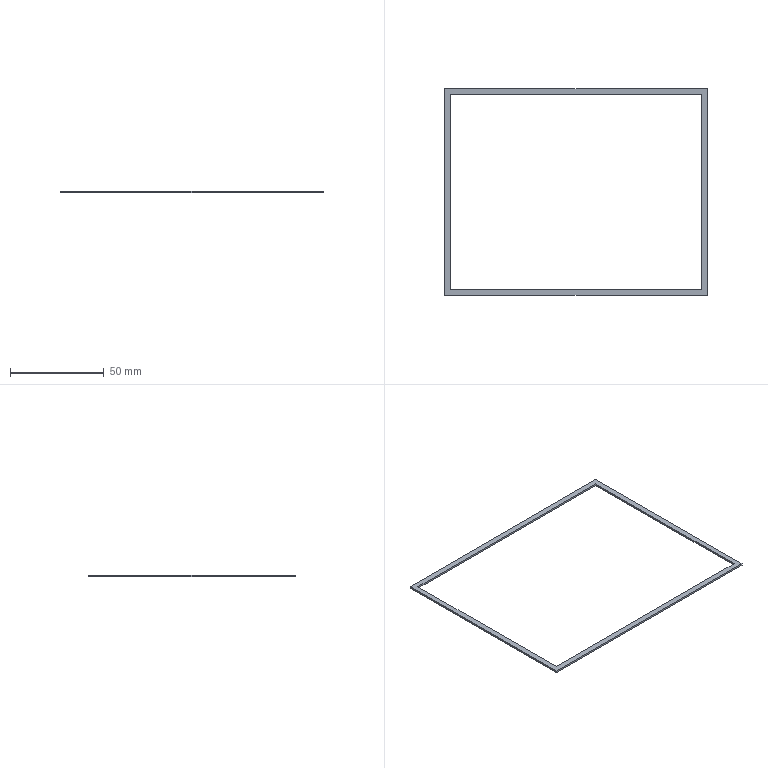Part | SolidWorks | features Extrusion 1 | 1 solid | 10 faces | box 140 x 110 x 1 mm | volume 1464 mm3 | plane 10
STEP:
#1=CARTESIAN_POINT('',(-70.,55.,0.5));
#2=VERTEX_POINT('',#1);
#3=CARTESIAN_POINT('',(-70.,-55.,0.5));
#4=VERTEX_POINT('',#3);
#5=CARTESIAN_POINT('',(-70.,55.,0.5));
#6=DIRECTION('',(0.,-1.,0.));
#7=VECTOR('',#6,1000.);
#8=LINE('',#5,#7);
#9=EDGE_CURVE('',#2,#4,#8,.T.);
#10=ORIENTED_EDGE('',*,*,#9,.F.);
#11=CARTESIAN_POINT('',(-70.,55.,-0.5));
#12=VERTEX_POINT('',#11);
#13=CARTESIAN_POINT('',(-70.,55.,-0.5));
#14=DIRECTION('',(0.,0.,1.));
#15=VECTOR('',#14,1000.);
#16=LINE('',#13,#15);
#17=EDGE_CURVE('',#12,#2,#16,.T.);
#18=ORIENTED_EDGE('',*,*,#17,.F.);
#19=CARTESIAN_POINT('',(-70.,-55.,-0.5));
#20=VERTEX_POINT('',#19);
#21=CARTESIAN_POINT('',(-70.,55.,-0.5));
#22=DIRECTION('',(0.,-1.,0.));
#23=VECTOR('',#22,1000.);
#24=LINE('',#21,#23);
#25=EDGE_CURVE('',#12,#20,#24,.T.);
#26=ORIENTED_EDGE('',*,*,#25,.T.);
#27=CARTESIAN_POINT('',(-70.,-55.,-0.5));
#28=DIRECTION('',(0.,0.,1.));
#29=VECTOR('',#28,1000.);
#30=LINE('',#27,#29);
#31=EDGE_CURVE('',#20,#4,#30,.T.);
#32=ORIENTED_EDGE('',*,*,#31,.T.);
#33=EDGE_LOOP('',(#10,#18,#26,#32));
#34=FACE_OUTER_BOUND('',#33,.T.);
#35=CARTESIAN_POINT('',(-70.,55.,-0.5));
#36=DIRECTION('',(-1.,0.,0.));
#37=DIRECTION('',(0.,0.,1.));
#38=AXIS2_PLACEMENT_3D('',#35,#36,#37);
#39=PLANE('',#38);
#40=ADVANCED_FACE('',(#34),#39,.T.);
#41=CARTESIAN_POINT('',(70.,55.,0.5));
#42=VERTEX_POINT('',#41);
#43=CARTESIAN_POINT('',(70.,55.,0.5));
#44=DIRECTION('',(-1.,0.,0.));
#45=VECTOR('',#44,1000.);
#46=LINE('',#43,#45);
#47=EDGE_CURVE('',#42,#2,#46,.T.);
#48=ORIENTED_EDGE('',*,*,#47,.F.);
#49=CARTESIAN_POINT('',(70.,55.,-0.5));
#50=VERTEX_POINT('',#49);
#51=CARTESIAN_POINT('',(70.,55.,-0.5));
#52=DIRECTION('',(0.,0.,1.));
#53=VECTOR('',#52,1000.);
#54=LINE('',#51,#53);
#55=EDGE_CURVE('',#50,#42,#54,.T.);
#56=ORIENTED_EDGE('',*,*,#55,.F.);
#57=CARTESIAN_POINT('',(70.,55.,-0.5));
#58=DIRECTION('',(-1.,0.,0.));
#59=VECTOR('',#58,1000.);
#60=LINE('',#57,#59);
#61=EDGE_CURVE('',#50,#12,#60,.T.);
#62=ORIENTED_EDGE('',*,*,#61,.T.);
#63=ORIENTED_EDGE('',*,*,#17,.T.);
#64=EDGE_LOOP('',(#48,#56,#62,#63));
#65=FACE_OUTER_BOUND('',#64,.T.);
#66=CARTESIAN_POINT('',(70.,55.,-0.5));
#67=DIRECTION('',(0.,1.,0.));
#68=DIRECTION('',(0.,0.,1.));
#69=AXIS2_PLACEMENT_3D('',#66,#67,#68);
#70=PLANE('',#69);
#71=ADVANCED_FACE('',(#65),#70,.T.);
#72=CARTESIAN_POINT('',(70.,-55.,0.5));
#73=VERTEX_POINT('',#72);
#74=CARTESIAN_POINT('',(70.,-55.,0.5));
#75=DIRECTION('',(0.,1.,0.));
#76=VECTOR('',#75,1000.);
#77=LINE('',#74,#76);
#78=EDGE_CURVE('',#73,#42,#77,.T.);
#79=ORIENTED_EDGE('',*,*,#78,.F.);
#80=CARTESIAN_POINT('',(70.,-55.,-0.5));
#81=VERTEX_POINT('',#80);
#82=CARTESIAN_POINT('',(70.,-55.,-0.5));
#83=DIRECTION('',(0.,0.,1.));
#84=VECTOR('',#83,1000.);
#85=LINE('',#82,#84);
#86=EDGE_CURVE('',#81,#73,#85,.T.);
#87=ORIENTED_EDGE('',*,*,#86,.F.);
#88=CARTESIAN_POINT('',(70.,-55.,-0.5));
#89=DIRECTION('',(0.,1.,0.));
#90=VECTOR('',#89,1000.);
#91=LINE('',#88,#90);
#92=EDGE_CURVE('',#81,#50,#91,.T.);
#93=ORIENTED_EDGE('',*,*,#92,.T.);
#94=ORIENTED_EDGE('',*,*,#55,.T.);
#95=EDGE_LOOP('',(#79,#87,#93,#94));
#96=FACE_OUTER_BOUND('',#95,.T.);
#97=CARTESIAN_POINT('',(70.,-55.,-0.5));
#98=DIRECTION('',(1.,0.,0.));
#99=DIRECTION('',(0.,0.,-1.));
#100=AXIS2_PLACEMENT_3D('',#97,#98,#99);
#101=PLANE('',#100);
#102=ADVANCED_FACE('',(#96),#101,.T.);
#103=CARTESIAN_POINT('',(-70.,-55.,0.5));
#104=DIRECTION('',(1.,0.,0.));
#105=VECTOR('',#104,1000.);
#106=LINE('',#103,#105);
#107=EDGE_CURVE('',#4,#73,#106,.T.);
#108=ORIENTED_EDGE('',*,*,#107,.F.);
#109=ORIENTED_EDGE('',*,*,#31,.F.);
#110=CARTESIAN_POINT('',(-70.,-55.,-0.5));
#111=DIRECTION('',(1.,0.,0.));
#112=VECTOR('',#111,1000.);
#113=LINE('',#110,#112);
#114=EDGE_CURVE('',#20,#81,#113,.T.);
#115=ORIENTED_EDGE('',*,*,#114,.T.);
#116=ORIENTED_EDGE('',*,*,#86,.T.);
#117=EDGE_LOOP('',(#108,#109,#115,#116));
#118=FACE_OUTER_BOUND('',#117,.T.);
#119=CARTESIAN_POINT('',(-70.,-55.,-0.5));
#120=DIRECTION('',(0.,-1.,0.));
#121=DIRECTION('',(0.,0.,-1.));
#122=AXIS2_PLACEMENT_3D('',#119,#120,#121);
#123=PLANE('',#122);
#124=ADVANCED_FACE('',(#118),#123,.T.);
#125=CARTESIAN_POINT('',(67.,52.,-0.5));
#126=VERTEX_POINT('',#125);
#127=CARTESIAN_POINT('',(-67.,52.,-0.5));
#128=VERTEX_POINT('',#127);
#129=CARTESIAN_POINT('',(67.,52.,-0.5));
#130=DIRECTION('',(-1.,0.,0.));
#131=VECTOR('',#130,1000.);
#132=LINE('',#129,#131);
#133=EDGE_CURVE('',#126,#128,#132,.T.);
#134=ORIENTED_EDGE('',*,*,#133,.T.);
#135=CARTESIAN_POINT('',(-67.,-52.,-0.5));
#136=VERTEX_POINT('',#135);
#137=CARTESIAN_POINT('',(-67.,52.,-0.5));
#138=DIRECTION('',(0.,-1.,0.));
#139=VECTOR('',#138,1000.);
#140=LINE('',#137,#139);
#141=EDGE_CURVE('',#128,#136,#140,.T.);
#142=ORIENTED_EDGE('',*,*,#141,.T.);
#143=CARTESIAN_POINT('',(67.,-52.,-0.5));
#144=VERTEX_POINT('',#143);
#145=CARTESIAN_POINT('',(-67.,-52.,-0.5));
#146=DIRECTION('',(1.,0.,0.));
#147=VECTOR('',#146,1000.);
#148=LINE('',#145,#147);
#149=EDGE_CURVE('',#136,#144,#148,.T.);
#150=ORIENTED_EDGE('',*,*,#149,.T.);
#151=CARTESIAN_POINT('',(67.,-52.,-0.5));
#152=DIRECTION('',(0.,1.,0.));
#153=VECTOR('',#152,1000.);
#154=LINE('',#151,#153);
#155=EDGE_CURVE('',#144,#126,#154,.T.);
#156=ORIENTED_EDGE('',*,*,#155,.T.);
#157=EDGE_LOOP('',(#134,#142,#150,#156));
#158=FACE_BOUND('',#157,.T.);
#159=ORIENTED_EDGE('',*,*,#25,.F.);
#160=ORIENTED_EDGE('',*,*,#61,.F.);
#161=ORIENTED_EDGE('',*,*,#92,.F.);
#162=ORIENTED_EDGE('',*,*,#114,.F.);
#163=EDGE_LOOP('',(#159,#160,#161,#162));
#164=FACE_OUTER_BOUND('',#163,.T.);
#165=CARTESIAN_POINT('',(0.,0.,-0.5));
#166=DIRECTION('',(0.,0.,1.));
#167=DIRECTION('',(1.,0.,0.));
#168=AXIS2_PLACEMENT_3D('',#165,#166,#167);
#169=PLANE('',#168);
#170=ADVANCED_FACE('',(#158,#164),#169,.F.);
#171=CARTESIAN_POINT('',(-67.,52.,0.5));
#172=VERTEX_POINT('',#171);
#173=CARTESIAN_POINT('',(-67.,-52.,0.5));
#174=VERTEX_POINT('',#173);
#175=CARTESIAN_POINT('',(-67.,52.,0.5));
#176=DIRECTION('',(0.,-1.,0.));
#177=VECTOR('',#176,1000.);
#178=LINE('',#175,#177);
#179=EDGE_CURVE('',#172,#174,#178,.T.);
#180=ORIENTED_EDGE('',*,*,#179,.F.);
#181=CARTESIAN_POINT('',(67.,52.,0.5));
#182=VERTEX_POINT('',#181);
#183=CARTESIAN_POINT('',(67.,52.,0.5));
#184=DIRECTION('',(-1.,0.,0.));
#185=VECTOR('',#184,1000.);
#186=LINE('',#183,#185);
#187=EDGE_CURVE('',#182,#172,#186,.T.);
#188=ORIENTED_EDGE('',*,*,#187,.F.);
#189=CARTESIAN_POINT('',(67.,-52.,0.5));
#190=VERTEX_POINT('',#189);
#191=CARTESIAN_POINT('',(67.,-52.,0.5));
#192=DIRECTION('',(0.,1.,0.));
#193=VECTOR('',#192,1000.);
#194=LINE('',#191,#193);
#195=EDGE_CURVE('',#190,#182,#194,.T.);
#196=ORIENTED_EDGE('',*,*,#195,.F.);
#197=CARTESIAN_POINT('',(-67.,-52.,0.5));
#198=DIRECTION('',(1.,0.,0.));
#199=VECTOR('',#198,1000.);
#200=LINE('',#197,#199);
#201=EDGE_CURVE('',#174,#190,#200,.T.);
#202=ORIENTED_EDGE('',*,*,#201,.F.);
#203=EDGE_LOOP('',(#180,#188,#196,#202));
#204=FACE_BOUND('',#203,.T.);
#205=ORIENTED_EDGE('',*,*,#9,.T.);
#206=ORIENTED_EDGE('',*,*,#107,.T.);
#207=ORIENTED_EDGE('',*,*,#78,.T.);
#208=ORIENTED_EDGE('',*,*,#47,.T.);
#209=EDGE_LOOP('',(#205,#206,#207,#208));
#210=FACE_OUTER_BOUND('',#209,.T.);
#211=CARTESIAN_POINT('',(0.,0.,0.5));
#212=DIRECTION('',(0.,0.,1.));
#213=DIRECTION('',(1.,0.,0.));
#214=AXIS2_PLACEMENT_3D('',#211,#212,#213);
#215=PLANE('',#214);
#216=ADVANCED_FACE('',(#204,#210),#215,.T.);
#217=ORIENTED_EDGE('',*,*,#179,.T.);
#218=CARTESIAN_POINT('',(-67.,-52.,-0.5));
#219=DIRECTION('',(0.,0.,1.));
#220=VECTOR('',#219,1000.);
#221=LINE('',#218,#220);
#222=EDGE_CURVE('',#136,#174,#221,.T.);
#223=ORIENTED_EDGE('',*,*,#222,.F.);
#224=ORIENTED_EDGE('',*,*,#141,.F.);
#225=CARTESIAN_POINT('',(-67.,52.,-0.5));
#226=DIRECTION('',(0.,0.,1.));
#227=VECTOR('',#226,1000.);
#228=LINE('',#225,#227);
#229=EDGE_CURVE('',#128,#172,#228,.T.);
#230=ORIENTED_EDGE('',*,*,#229,.T.);
#231=EDGE_LOOP('',(#217,#223,#224,#230));
#232=FACE_OUTER_BOUND('',#231,.T.);
#233=CARTESIAN_POINT('',(-67.,52.,-0.5));
#234=DIRECTION('',(-1.,0.,0.));
#235=DIRECTION('',(0.,0.,1.));
#236=AXIS2_PLACEMENT_3D('',#233,#234,#235);
#237=PLANE('',#236);
#238=ADVANCED_FACE('',(#232),#237,.F.);
#239=ORIENTED_EDGE('',*,*,#187,.T.);
#240=ORIENTED_EDGE('',*,*,#229,.F.);
#241=ORIENTED_EDGE('',*,*,#133,.F.);
#242=CARTESIAN_POINT('',(67.,52.,-0.5));
#243=DIRECTION('',(0.,0.,1.));
#244=VECTOR('',#243,1000.);
#245=LINE('',#242,#244);
#246=EDGE_CURVE('',#126,#182,#245,.T.);
#247=ORIENTED_EDGE('',*,*,#246,.T.);
#248=EDGE_LOOP('',(#239,#240,#241,#247));
#249=FACE_OUTER_BOUND('',#248,.T.);
#250=CARTESIAN_POINT('',(67.,52.,-0.5));
#251=DIRECTION('',(0.,1.,0.));
#252=DIRECTION('',(0.,0.,1.));
#253=AXIS2_PLACEMENT_3D('',#250,#251,#252);
#254=PLANE('',#253);
#255=ADVANCED_FACE('',(#249),#254,.F.);
#256=ORIENTED_EDGE('',*,*,#195,.T.);
#257=ORIENTED_EDGE('',*,*,#246,.F.);
#258=ORIENTED_EDGE('',*,*,#155,.F.);
#259=CARTESIAN_POINT('',(67.,-52.,-0.5));
#260=DIRECTION('',(0.,0.,1.));
#261=VECTOR('',#260,1000.);
#262=LINE('',#259,#261);
#263=EDGE_CURVE('',#144,#190,#262,.T.);
#264=ORIENTED_EDGE('',*,*,#263,.T.);
#265=EDGE_LOOP('',(#256,#257,#258,#264));
#266=FACE_OUTER_BOUND('',#265,.T.);
#267=CARTESIAN_POINT('',(67.,-52.,-0.5));
#268=DIRECTION('',(1.,0.,0.));
#269=DIRECTION('',(0.,0.,-1.));
#270=AXIS2_PLACEMENT_3D('',#267,#268,#269);
#271=PLANE('',#270);
#272=ADVANCED_FACE('',(#266),#271,.F.);
#273=ORIENTED_EDGE('',*,*,#201,.T.);
#274=ORIENTED_EDGE('',*,*,#263,.F.);
#275=ORIENTED_EDGE('',*,*,#149,.F.);
#276=ORIENTED_EDGE('',*,*,#222,.T.);
#277=EDGE_LOOP('',(#273,#274,#275,#276));
#278=FACE_OUTER_BOUND('',#277,.T.);
#279=CARTESIAN_POINT('',(-67.,-52.,-0.5));
#280=DIRECTION('',(0.,-1.,0.));
#281=DIRECTION('',(0.,0.,-1.));
#282=AXIS2_PLACEMENT_3D('',#279,#280,#281);
#283=PLANE('',#282);
#284=ADVANCED_FACE('',(#278),#283,.F.);
#285=CLOSED_SHELL('',(#40,#71,#102,#124,#170,#216,#238,#255,#272,#284));
#286=MANIFOLD_SOLID_BREP('',#285);
#287=CARTESIAN_POINT('',(0.,0.,0.));
#288=DIRECTION('',(0.,0.,1.));
#289=DIRECTION('',(1.,0.,0.));
#290=AXIS2_PLACEMENT_3D('',#287,#288,#289);
#291=(LENGTH_UNIT()NAMED_UNIT(*)SI_UNIT(.MILLI.,.METRE.));
#292=UNCERTAINTY_MEASURE_WITH_UNIT(LENGTH_MEASURE(0.00001),#291,'','');
#293=(NAMED_UNIT(*)PLANE_ANGLE_UNIT()SI_UNIT($,.RADIAN.));
#294=(NAMED_UNIT(*)SI_UNIT($,.STERADIAN.)SOLID_ANGLE_UNIT());
#295=(GEOMETRIC_REPRESENTATION_CONTEXT(3)GLOBAL_UNCERTAINTY_ASSIGNED_CONTEXT((#292))GLOBAL_UNIT_ASSIGNED_CONTEXT((#291,#293,#294))REPRESENTATION_CONTEXT('',''));
#296=ADVANCED_BREP_SHAPE_REPRESENTATION('',(#286,#290),#295);